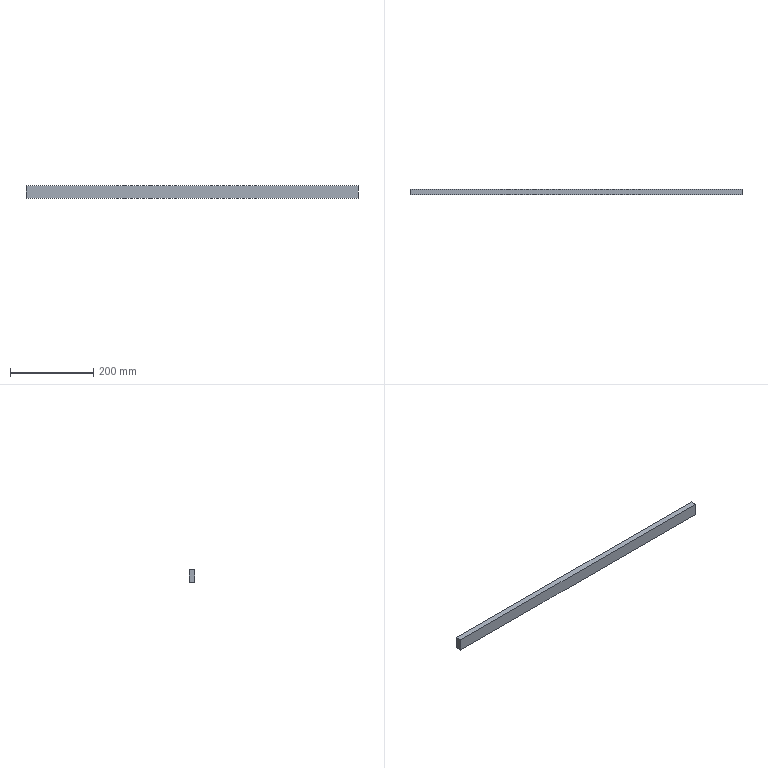Part | SolidWorks | features Extrusion 1 | 1 solid | 6 faces | box 800 x 14 x 30 mm | volume 336000 mm3 | plane 6
STEP:
#1=CARTESIAN_POINT('',(400.,-7.,0.));
#2=VERTEX_POINT('',#1);
#3=CARTESIAN_POINT('',(400.,7.,0.));
#4=VERTEX_POINT('',#3);
#5=CARTESIAN_POINT('',(400.,-7.,0.));
#6=DIRECTION('',(0.,1.,0.));
#7=VECTOR('',#6,1000.);
#8=LINE('',#5,#7);
#9=EDGE_CURVE('',#2,#4,#8,.T.);
#10=ORIENTED_EDGE('',*,*,#9,.T.);
#11=CARTESIAN_POINT('',(400.,7.,30.));
#12=VERTEX_POINT('',#11);
#13=CARTESIAN_POINT('',(400.,7.,30.));
#14=DIRECTION('',(0.,0.,-1.));
#15=VECTOR('',#14,1000.);
#16=LINE('',#13,#15);
#17=EDGE_CURVE('',#12,#4,#16,.T.);
#18=ORIENTED_EDGE('',*,*,#17,.F.);
#19=CARTESIAN_POINT('',(400.,-7.,30.));
#20=VERTEX_POINT('',#19);
#21=CARTESIAN_POINT('',(400.,-7.,30.));
#22=DIRECTION('',(0.,1.,0.));
#23=VECTOR('',#22,1000.);
#24=LINE('',#21,#23);
#25=EDGE_CURVE('',#20,#12,#24,.T.);
#26=ORIENTED_EDGE('',*,*,#25,.F.);
#27=CARTESIAN_POINT('',(400.,-7.,30.));
#28=DIRECTION('',(0.,0.,-1.));
#29=VECTOR('',#28,1000.);
#30=LINE('',#27,#29);
#31=EDGE_CURVE('',#20,#2,#30,.T.);
#32=ORIENTED_EDGE('',*,*,#31,.T.);
#33=EDGE_LOOP('',(#10,#18,#26,#32));
#34=FACE_OUTER_BOUND('',#33,.T.);
#35=CARTESIAN_POINT('',(400.,-7.,30.));
#36=DIRECTION('',(-1.,0.,0.));
#37=DIRECTION('',(0.,0.,1.));
#38=AXIS2_PLACEMENT_3D('',#35,#36,#37);
#39=PLANE('',#38);
#40=ADVANCED_FACE('',(#34),#39,.F.);
#41=CARTESIAN_POINT('',(-400.,7.,0.));
#42=VERTEX_POINT('',#41);
#43=CARTESIAN_POINT('',(-400.,7.,0.));
#44=DIRECTION('',(-1.,0.,0.));
#45=VECTOR('',#44,1000.);
#46=LINE('',#43,#45);
#47=EDGE_CURVE('',#4,#42,#46,.T.);
#48=ORIENTED_EDGE('',*,*,#47,.T.);
#49=CARTESIAN_POINT('',(-400.,7.,30.));
#50=VERTEX_POINT('',#49);
#51=CARTESIAN_POINT('',(-400.,7.,30.));
#52=DIRECTION('',(0.,0.,-1.));
#53=VECTOR('',#52,1000.);
#54=LINE('',#51,#53);
#55=EDGE_CURVE('',#50,#42,#54,.T.);
#56=ORIENTED_EDGE('',*,*,#55,.F.);
#57=CARTESIAN_POINT('',(-400.,7.,30.));
#58=DIRECTION('',(-1.,0.,0.));
#59=VECTOR('',#58,1000.);
#60=LINE('',#57,#59);
#61=EDGE_CURVE('',#12,#50,#60,.T.);
#62=ORIENTED_EDGE('',*,*,#61,.F.);
#63=ORIENTED_EDGE('',*,*,#17,.T.);
#64=EDGE_LOOP('',(#48,#56,#62,#63));
#65=FACE_OUTER_BOUND('',#64,.T.);
#66=CARTESIAN_POINT('',(-400.,7.,30.));
#67=DIRECTION('',(0.,-1.,0.));
#68=DIRECTION('',(0.,0.,-1.));
#69=AXIS2_PLACEMENT_3D('',#66,#67,#68);
#70=PLANE('',#69);
#71=ADVANCED_FACE('',(#65),#70,.F.);
#72=CARTESIAN_POINT('',(-400.,-7.,0.));
#73=VERTEX_POINT('',#72);
#74=CARTESIAN_POINT('',(-400.,-7.,0.));
#75=DIRECTION('',(0.,-1.,0.));
#76=VECTOR('',#75,1000.);
#77=LINE('',#74,#76);
#78=EDGE_CURVE('',#42,#73,#77,.T.);
#79=ORIENTED_EDGE('',*,*,#78,.T.);
#80=CARTESIAN_POINT('',(-400.,-7.,30.));
#81=VERTEX_POINT('',#80);
#82=CARTESIAN_POINT('',(-400.,-7.,30.));
#83=DIRECTION('',(0.,0.,-1.));
#84=VECTOR('',#83,1000.);
#85=LINE('',#82,#84);
#86=EDGE_CURVE('',#81,#73,#85,.T.);
#87=ORIENTED_EDGE('',*,*,#86,.F.);
#88=CARTESIAN_POINT('',(-400.,-7.,30.));
#89=DIRECTION('',(0.,-1.,0.));
#90=VECTOR('',#89,1000.);
#91=LINE('',#88,#90);
#92=EDGE_CURVE('',#50,#81,#91,.T.);
#93=ORIENTED_EDGE('',*,*,#92,.F.);
#94=ORIENTED_EDGE('',*,*,#55,.T.);
#95=EDGE_LOOP('',(#79,#87,#93,#94));
#96=FACE_OUTER_BOUND('',#95,.T.);
#97=CARTESIAN_POINT('',(-400.,-7.,30.));
#98=DIRECTION('',(1.,0.,0.));
#99=DIRECTION('',(0.,0.,-1.));
#100=AXIS2_PLACEMENT_3D('',#97,#98,#99);
#101=PLANE('',#100);
#102=ADVANCED_FACE('',(#96),#101,.F.);
#103=CARTESIAN_POINT('',(-400.,-7.,0.));
#104=DIRECTION('',(1.,0.,0.));
#105=VECTOR('',#104,1000.);
#106=LINE('',#103,#105);
#107=EDGE_CURVE('',#73,#2,#106,.T.);
#108=ORIENTED_EDGE('',*,*,#107,.T.);
#109=ORIENTED_EDGE('',*,*,#31,.F.);
#110=CARTESIAN_POINT('',(-400.,-7.,30.));
#111=DIRECTION('',(1.,0.,0.));
#112=VECTOR('',#111,1000.);
#113=LINE('',#110,#112);
#114=EDGE_CURVE('',#81,#20,#113,.T.);
#115=ORIENTED_EDGE('',*,*,#114,.F.);
#116=ORIENTED_EDGE('',*,*,#86,.T.);
#117=EDGE_LOOP('',(#108,#109,#115,#116));
#118=FACE_OUTER_BOUND('',#117,.T.);
#119=CARTESIAN_POINT('',(-400.,-7.,30.));
#120=DIRECTION('',(0.,1.,0.));
#121=DIRECTION('',(0.,0.,1.));
#122=AXIS2_PLACEMENT_3D('',#119,#120,#121);
#123=PLANE('',#122);
#124=ADVANCED_FACE('',(#118),#123,.F.);
#125=ORIENTED_EDGE('',*,*,#25,.T.);
#126=ORIENTED_EDGE('',*,*,#61,.T.);
#127=ORIENTED_EDGE('',*,*,#92,.T.);
#128=ORIENTED_EDGE('',*,*,#114,.T.);
#129=EDGE_LOOP('',(#125,#126,#127,#128));
#130=FACE_OUTER_BOUND('',#129,.T.);
#131=CARTESIAN_POINT('',(0.,0.,30.));
#132=DIRECTION('',(0.,0.,-1.));
#133=DIRECTION('',(-1.,0.,0.));
#134=AXIS2_PLACEMENT_3D('',#131,#132,#133);
#135=PLANE('',#134);
#136=ADVANCED_FACE('',(#130),#135,.F.);
#137=ORIENTED_EDGE('',*,*,#9,.F.);
#138=ORIENTED_EDGE('',*,*,#107,.F.);
#139=ORIENTED_EDGE('',*,*,#78,.F.);
#140=ORIENTED_EDGE('',*,*,#47,.F.);
#141=EDGE_LOOP('',(#137,#138,#139,#140));
#142=FACE_OUTER_BOUND('',#141,.T.);
#143=CARTESIAN_POINT('',(0.,0.,0.));
#144=DIRECTION('',(0.,0.,-1.));
#145=DIRECTION('',(-1.,0.,0.));
#146=AXIS2_PLACEMENT_3D('',#143,#144,#145);
#147=PLANE('',#146);
#148=ADVANCED_FACE('',(#142),#147,.T.);
#149=CLOSED_SHELL('',(#40,#71,#102,#124,#136,#148));
#150=MANIFOLD_SOLID_BREP('',#149);
#151=CARTESIAN_POINT('',(0.,0.,0.));
#152=DIRECTION('',(0.,0.,1.));
#153=DIRECTION('',(1.,0.,0.));
#154=AXIS2_PLACEMENT_3D('',#151,#152,#153);
#155=(LENGTH_UNIT()NAMED_UNIT(*)SI_UNIT(.MILLI.,.METRE.));
#156=UNCERTAINTY_MEASURE_WITH_UNIT(LENGTH_MEASURE(0.00001),#155,'','');
#157=(NAMED_UNIT(*)PLANE_ANGLE_UNIT()SI_UNIT($,.RADIAN.));
#158=(NAMED_UNIT(*)SI_UNIT($,.STERADIAN.)SOLID_ANGLE_UNIT());
#159=(GEOMETRIC_REPRESENTATION_CONTEXT(3)GLOBAL_UNCERTAINTY_ASSIGNED_CONTEXT((#156))GLOBAL_UNIT_ASSIGNED_CONTEXT((#155,#157,#158))REPRESENTATION_CONTEXT('',''));
#160=ADVANCED_BREP_SHAPE_REPRESENTATION('',(#150,#154),#159);